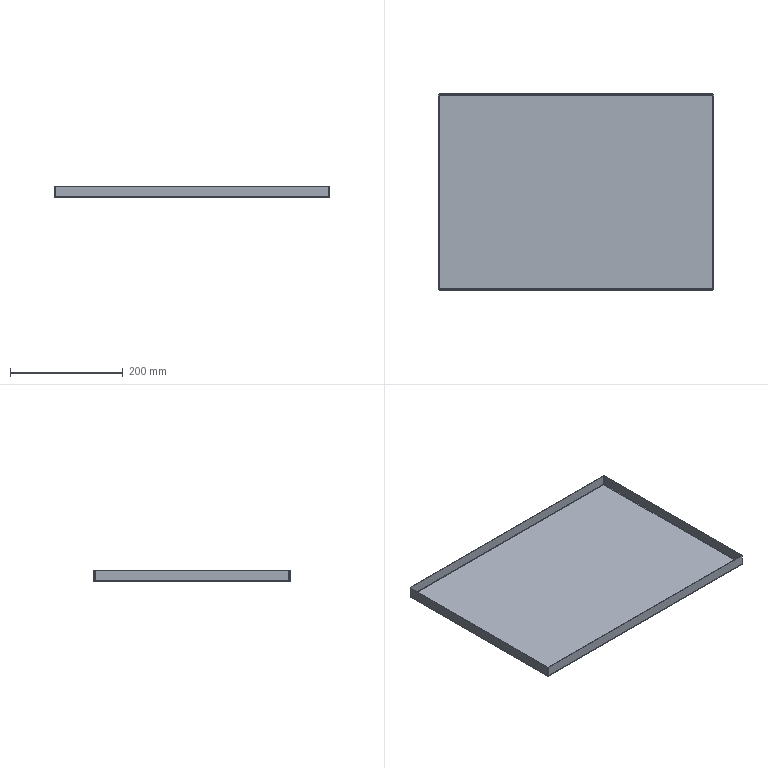Part | STEP file | X77-03007 | 1 solid | 38 faces | box 488 x 348 x 20 mm | volume 299031 mm3 | plane 22 | spline 8 | cylinder 8 | commonest cylinder face diameters 1.473 x4 4.473 x4